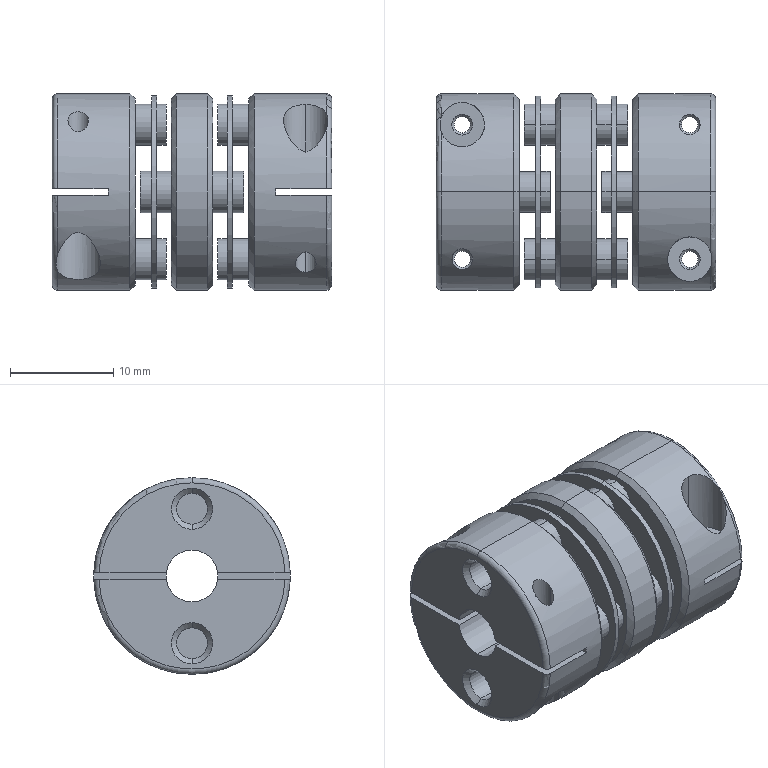Part | NX | features BREP 1 | 1 solid | 170 faces | box 27 x 19 x 19 mm | volume 4748 mm3 | cylinder 92 | plane 40 | cone 32 | torus 6 | commonest cylinder face diameters 4 x32 2 x16 1.567 x8 3 x8 4.3 x8 8.5 x6